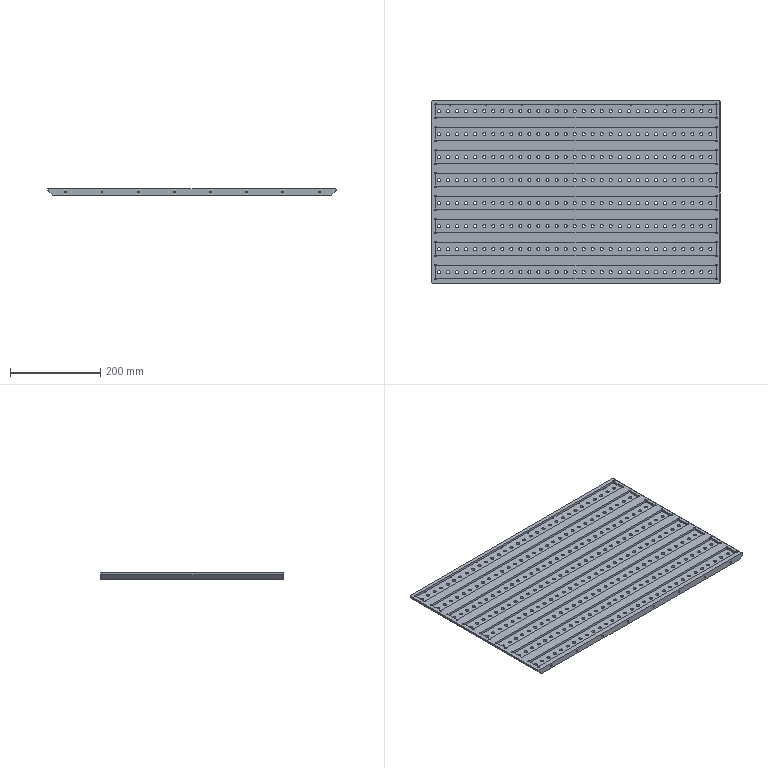Part | STEP file | PN_0012 | 1 solid | 661 faces | box 638 x 404 x 14 mm | volume 2739092 mm3 | cylinder 577 | plane 52 | cone 32 | commonest cylinder face diameters 6.8 x496 4 x49 4.2 x32